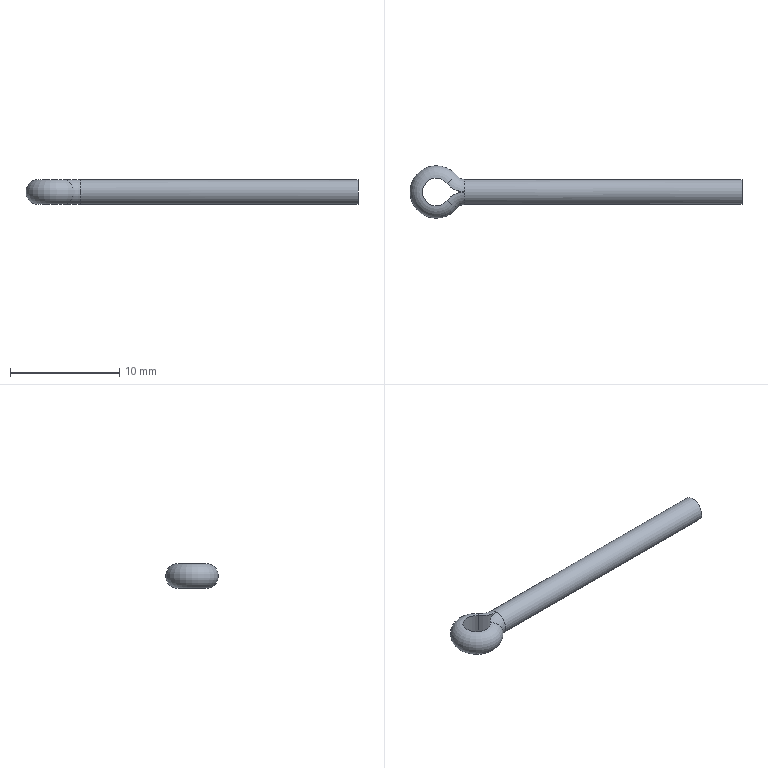Part | NX | features solid 2 | 1 solid | 8 faces | box 30.416 x 4.826 x 2.286 mm | volume 127.87 mm3 | cylinder 4 | torus 3 | plane 1 | commonest cylinder face diameters 4.064 x2 2.286 x1 2.54 x1
STEP:
#1=CARTESIAN_POINT('',(-27.002,-0.7815,-1.143));
#2=VERTEX_POINT('',#1);
#3=CARTESIAN_POINT('',(-27.002,-0.7815,1.143));
#4=VERTEX_POINT('',#3);
#5=CARTESIAN_POINT('',(-27.002,-0.7815,-1.143));
#6=DIRECTION('',(0.,0.,1.));
#7=VECTOR('',#6,1000.);
#8=LINE('',#5,#7);
#9=EDGE_CURVE('',#2,#4,#8,.T.);
#10=ORIENTED_EDGE('',*,*,#9,.F.);
#11=CARTESIAN_POINT('',(-27.002,0.7815,-1.143));
#12=VERTEX_POINT('',#11);
#13=CARTESIAN_POINT('',(-28.003,0.,-1.143));
#14=DIRECTION('',(0.,0.,-1.));
#15=DIRECTION('',(-1.,0.,0.));
#16=AXIS2_PLACEMENT_3D('',#13,#14,#15);
#17=CIRCLE('',#16,1.27);
#18=EDGE_CURVE('',#2,#12,#17,.T.);
#19=ORIENTED_EDGE('',*,*,#18,.T.);
#20=CARTESIAN_POINT('',(-27.002,0.7815,1.143));
#21=VERTEX_POINT('',#20);
#22=CARTESIAN_POINT('',(-27.002,0.7815,-1.143));
#23=DIRECTION('',(0.,0.,1.));
#24=VECTOR('',#23,1000.);
#25=LINE('',#22,#24);
#26=EDGE_CURVE('',#12,#21,#25,.T.);
#27=ORIENTED_EDGE('',*,*,#26,.T.);
#28=CARTESIAN_POINT('',(-28.003,0.,1.143));
#29=DIRECTION('',(0.,0.,-1.));
#30=DIRECTION('',(-1.,0.,0.));
#31=AXIS2_PLACEMENT_3D('',#28,#29,#30);
#32=CIRCLE('',#31,1.27);
#33=EDGE_CURVE('',#21,#4,#32,.F.);
#34=ORIENTED_EDGE('',*,*,#33,.T.);
#35=EDGE_LOOP('',(#10,#19,#27,#34));
#36=FACE_BOUND('',#35,.T.);
#37=CARTESIAN_POINT('',(-28.003,0.,0.));
#38=DIRECTION('',(0.,0.,-1.));
#39=DIRECTION('',(-1.,0.,0.));
#40=AXIS2_PLACEMENT_3D('',#37,#38,#39);
#41=CYLINDRICAL_SURFACE('',#40,1.27);
#42=ADVANCED_FACE('',(#36),#41,.F.);
#43=CARTESIAN_POINT('',(-27.002,-0.7815,0.));
#44=DIRECTION('',(0.6154,0.7882,0.));
#45=DIRECTION('',(-0.7882,0.6154,0.));
#46=AXIS2_PLACEMENT_3D('',#43,#44,#45);
#47=CIRCLE('',#46,1.143);
#48=EDGE_CURVE('',#4,#2,#47,.T.);
#49=ORIENTED_EDGE('',*,*,#48,.F.);
#50=ORIENTED_EDGE('',*,*,#33,.F.);
#51=CARTESIAN_POINT('',(-27.002,0.7815,0.));
#52=DIRECTION('',(-0.6154,0.7882,0.));
#53=DIRECTION('',(-0.7882,-0.6154,0.));
#54=AXIS2_PLACEMENT_3D('',#51,#52,#53);
#55=CIRCLE('',#54,1.143);
#56=EDGE_CURVE('',#21,#12,#55,.T.);
#57=ORIENTED_EDGE('',*,*,#56,.T.);
#58=ORIENTED_EDGE('',*,*,#18,.F.);
#59=EDGE_LOOP('',(#49,#50,#57,#58));
#60=FACE_BOUND('',#59,.T.);
#61=CARTESIAN_POINT('',(-28.003,0.,0.));
#62=DIRECTION('',(0.,0.,-1.));
#63=DIRECTION('',(-1.,0.,0.));
#64=AXIS2_PLACEMENT_3D('',#61,#62,#63);
#65=TOROIDAL_SURFACE('',#64,1.27,1.143);
#66=ADVANCED_FACE('',(#60),#65,.T.);
#67=CARTESIAN_POINT('',(-25.4,0.,-1.143));
#68=VERTEX_POINT('',#67);
#69=CARTESIAN_POINT('',(-25.4,0.,1.143));
#70=VERTEX_POINT('',#69);
#71=CARTESIAN_POINT('',(-25.4,0.,-1.143));
#72=DIRECTION('',(0.,0.,1.));
#73=VECTOR('',#72,1000.);
#74=LINE('',#71,#73);
#75=EDGE_CURVE('',#68,#70,#74,.T.);
#76=ORIENTED_EDGE('',*,*,#75,.F.);
#77=CARTESIAN_POINT('',(-25.4,-2.032,-1.143));
#78=DIRECTION('',(0.,0.,1.));
#79=DIRECTION('',(1.,0.,0.));
#80=AXIS2_PLACEMENT_3D('',#77,#78,#79);
#81=CIRCLE('',#80,2.032);
#82=EDGE_CURVE('',#68,#2,#81,.T.);
#83=ORIENTED_EDGE('',*,*,#82,.T.);
#84=ORIENTED_EDGE('',*,*,#9,.T.);
#85=CARTESIAN_POINT('',(-25.4,-2.032,1.143));
#86=DIRECTION('',(0.,0.,1.));
#87=DIRECTION('',(1.,0.,0.));
#88=AXIS2_PLACEMENT_3D('',#85,#86,#87);
#89=CIRCLE('',#88,2.032);
#90=EDGE_CURVE('',#4,#70,#89,.F.);
#91=ORIENTED_EDGE('',*,*,#90,.T.);
#92=EDGE_LOOP('',(#76,#83,#84,#91));
#93=FACE_BOUND('',#92,.T.);
#94=CARTESIAN_POINT('',(-25.4,-2.032,0.));
#95=DIRECTION('',(0.,0.,1.));
#96=DIRECTION('',(1.,0.,0.));
#97=AXIS2_PLACEMENT_3D('',#94,#95,#96);
#98=CYLINDRICAL_SURFACE('',#97,2.032);
#99=ADVANCED_FACE('',(#93),#98,.T.);
#100=CARTESIAN_POINT('',(-25.4,0.,0.));
#101=DIRECTION('',(1.,0.,0.));
#102=DIRECTION('',(0.,1.,0.));
#103=AXIS2_PLACEMENT_3D('',#100,#101,#102);
#104=CIRCLE('',#103,1.143);
#105=EDGE_CURVE('',#70,#68,#104,.T.);
#106=ORIENTED_EDGE('',*,*,#105,.F.);
#107=ORIENTED_EDGE('',*,*,#90,.F.);
#108=ORIENTED_EDGE('',*,*,#48,.T.);
#109=ORIENTED_EDGE('',*,*,#82,.F.);
#110=EDGE_LOOP('',(#106,#107,#108,#109));
#111=FACE_BOUND('',#110,.T.);
#112=CARTESIAN_POINT('',(-25.4,-2.032,0.));
#113=DIRECTION('',(0.,0.,1.));
#114=DIRECTION('',(1.,0.,0.));
#115=AXIS2_PLACEMENT_3D('',#112,#113,#114);
#116=TOROIDAL_SURFACE('',#115,2.032,1.143);
#117=ADVANCED_FACE('',(#111),#116,.T.);
#118=CARTESIAN_POINT('',(0.,1.143,0.));
#119=VERTEX_POINT('',#118);
#120=CARTESIAN_POINT('',(0.,0.,0.));
#121=DIRECTION('',(1.,0.,0.));
#122=DIRECTION('',(0.,1.,0.));
#123=AXIS2_PLACEMENT_3D('',#120,#121,#122);
#124=CIRCLE('',#123,1.143);
#125=EDGE_CURVE('',#119,#119,#124,.T.);
#126=ORIENTED_EDGE('',*,*,#125,.F.);
#127=EDGE_LOOP('',(#126));
#128=FACE_BOUND('',#127,.T.);
#129=CARTESIAN_POINT('',(-25.4,0.,0.));
#130=DIRECTION('',(-1.,0.,0.));
#131=DIRECTION('',(0.,-1.,0.));
#132=AXIS2_PLACEMENT_3D('',#129,#130,#131);
#133=CIRCLE('',#132,1.143);
#134=EDGE_CURVE('',#68,#70,#133,.F.);
#135=ORIENTED_EDGE('',*,*,#134,.T.);
#136=ORIENTED_EDGE('',*,*,#105,.T.);
#137=EDGE_LOOP('',(#135,#136));
#138=FACE_BOUND('',#137,.T.);
#139=CARTESIAN_POINT('',(-25.4,0.,0.));
#140=DIRECTION('',(1.,0.,0.));
#141=DIRECTION('',(0.,0.,-1.));
#142=AXIS2_PLACEMENT_3D('',#139,#140,#141);
#143=CYLINDRICAL_SURFACE('',#142,1.143);
#144=ADVANCED_FACE('',(#128,#138),#143,.T.);
#145=ORIENTED_EDGE('',*,*,#125,.T.);
#146=EDGE_LOOP('',(#145));
#147=FACE_BOUND('',#146,.T.);
#148=CARTESIAN_POINT('',(0.,0.,0.));
#149=DIRECTION('',(1.,0.,0.));
#150=DIRECTION('',(0.,0.,-1.));
#151=AXIS2_PLACEMENT_3D('',#148,#149,#150);
#152=PLANE('',#151);
#153=ADVANCED_FACE('',(#147),#152,.T.);
#154=ORIENTED_EDGE('',*,*,#75,.T.);
#155=CARTESIAN_POINT('',(-25.4,2.032,1.143));
#156=DIRECTION('',(0.,0.,-1.));
#157=DIRECTION('',(1.,0.,0.));
#158=AXIS2_PLACEMENT_3D('',#155,#156,#157);
#159=CIRCLE('',#158,2.032);
#160=EDGE_CURVE('',#21,#70,#159,.F.);
#161=ORIENTED_EDGE('',*,*,#160,.F.);
#162=ORIENTED_EDGE('',*,*,#26,.F.);
#163=CARTESIAN_POINT('',(-25.4,2.032,-1.143));
#164=DIRECTION('',(0.,0.,-1.));
#165=DIRECTION('',(1.,0.,0.));
#166=AXIS2_PLACEMENT_3D('',#163,#164,#165);
#167=CIRCLE('',#166,2.032);
#168=EDGE_CURVE('',#68,#12,#167,.T.);
#169=ORIENTED_EDGE('',*,*,#168,.F.);
#170=EDGE_LOOP('',(#154,#161,#162,#169));
#171=FACE_BOUND('',#170,.T.);
#172=CARTESIAN_POINT('',(-25.4,2.032,0.));
#173=DIRECTION('',(0.,0.,1.));
#174=DIRECTION('',(1.,0.,0.));
#175=AXIS2_PLACEMENT_3D('',#172,#173,#174);
#176=CYLINDRICAL_SURFACE('',#175,2.032);
#177=ADVANCED_FACE('',(#171),#176,.T.);
#178=ORIENTED_EDGE('',*,*,#134,.F.);
#179=ORIENTED_EDGE('',*,*,#168,.T.);
#180=ORIENTED_EDGE('',*,*,#56,.F.);
#181=ORIENTED_EDGE('',*,*,#160,.T.);
#182=EDGE_LOOP('',(#178,#179,#180,#181));
#183=FACE_BOUND('',#182,.T.);
#184=CARTESIAN_POINT('',(-25.4,2.032,0.));
#185=DIRECTION('',(0.,0.,1.));
#186=DIRECTION('',(1.,0.,0.));
#187=AXIS2_PLACEMENT_3D('',#184,#185,#186);
#188=TOROIDAL_SURFACE('',#187,2.032,1.143);
#189=ADVANCED_FACE('',(#183),#188,.T.);
#190=CLOSED_SHELL('',(#42,#66,#99,#117,#144,#153,#177,#189));
#191=MANIFOLD_SOLID_BREP('',#190);
#192=(LENGTH_UNIT()NAMED_UNIT(*)SI_UNIT(.MILLI.,.METRE.));
#193=UNCERTAINTY_MEASURE_WITH_UNIT(LENGTH_MEASURE(0.00001),#192,'','');
#194=(NAMED_UNIT(*)PLANE_ANGLE_UNIT()SI_UNIT($,.RADIAN.));
#195=(NAMED_UNIT(*)SI_UNIT($,.STERADIAN.)SOLID_ANGLE_UNIT());
#196=(GEOMETRIC_REPRESENTATION_CONTEXT(3)GLOBAL_UNCERTAINTY_ASSIGNED_CONTEXT((#193))GLOBAL_UNIT_ASSIGNED_CONTEXT((#192,#194,#195))REPRESENTATION_CONTEXT('',''));
#197=ADVANCED_BREP_SHAPE_REPRESENTATION('',(#191),#196);